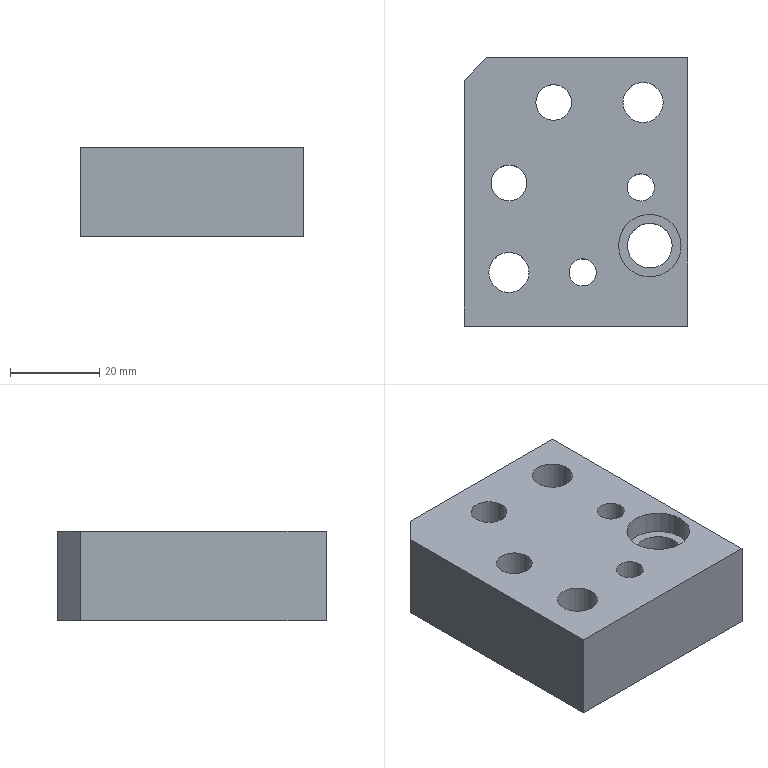Part | STEP file | 421_id2474_x_t | 1 solid | 24 faces | box 50 x 60 x 20 mm | volume 49706 mm3 | plane 12 | cylinder 12 | commonest cylinder face diameters 10 x3 14 x3 6.1 x2 8 x2 9 x2